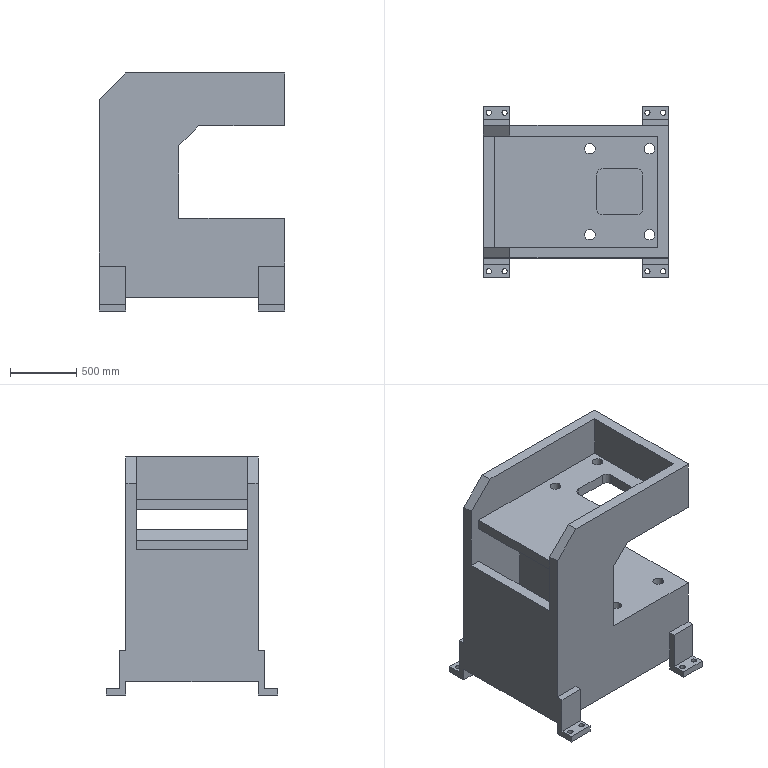Part | SolidWorks | features ICE 6, Chamfer 2, Cut 2, MirrorPattern 2, Extrusion 1, Fillet 1, MoveFace 1, Shell 1 | 1 solid | 93 faces | box 1400 x 1300 x 1800 mm | volume 599795931 mm3 | plane 57 | cylinder 36 | commonest cylinder face diameters 40 x16 80.2 x16 100 x4